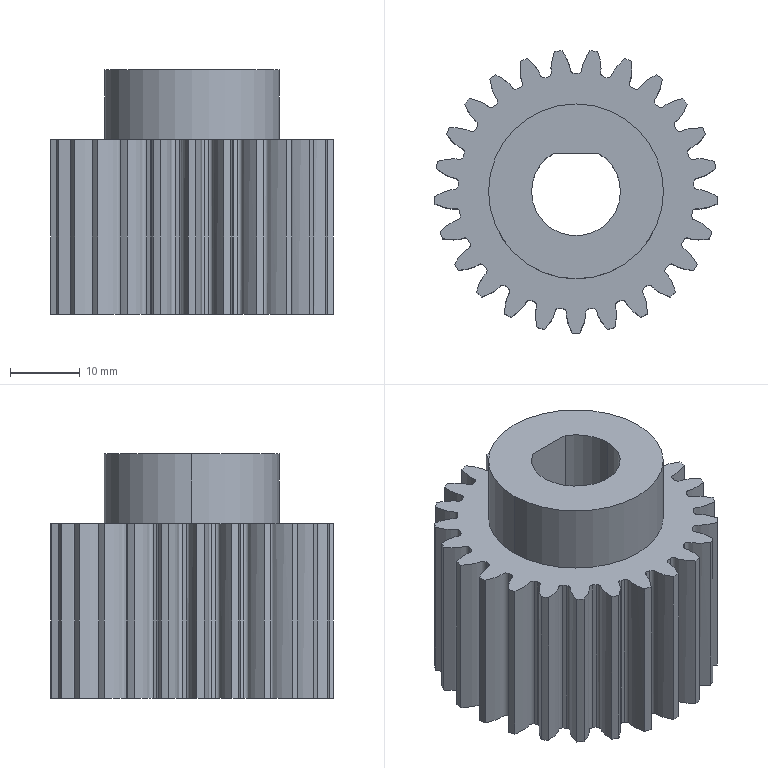Part | STEP file | X77-04010 | 1 solid | 109 faces | box 40.473 x 40.401 x 35 mm | volume 27750 mm3 | cylinder 55 | spline 50 | plane 4 | commonest cylinder face diameters 33.75 x25 40.5 x25 12.7 x3 25 x2